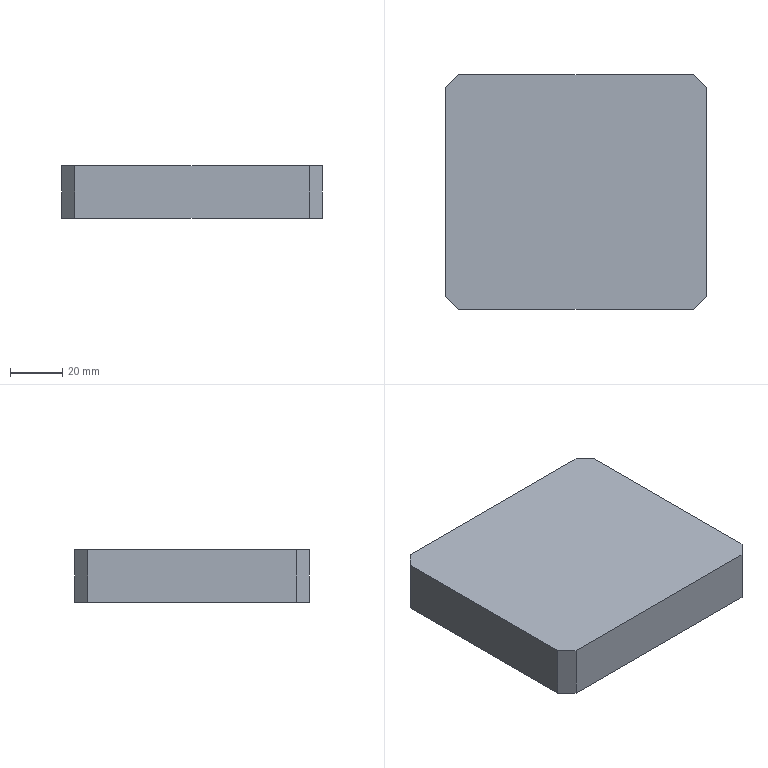Part | SolidWorks | features Chamfer 1, Extrusion 1 | 1 solid | 10 faces | box 100 x 90 x 20 mm | volume 179000 mm3 | plane 10
STEP:
#1=CARTESIAN_POINT('',(-46.616,42.258,0.));
#2=VERTEX_POINT('',#1);
#3=CARTESIAN_POINT('',(-46.616,-37.742,0.));
#4=VERTEX_POINT('',#3);
#5=CARTESIAN_POINT('',(-46.616,47.258,0.));
#6=DIRECTION('',(0.,-1.,0.));
#7=VECTOR('',#6,1000.);
#8=LINE('',#5,#7);
#9=EDGE_CURVE('',#2,#4,#8,.T.);
#10=ORIENTED_EDGE('',*,*,#9,.T.);
#11=CARTESIAN_POINT('',(-46.616,-37.742,20.));
#12=VERTEX_POINT('',#11);
#13=CARTESIAN_POINT('',(-46.616,-37.742,20.));
#14=DIRECTION('',(0.,0.,1.));
#15=VECTOR('',#14,1000.);
#16=LINE('',#13,#15);
#17=EDGE_CURVE('',#4,#12,#16,.T.);
#18=ORIENTED_EDGE('',*,*,#17,.T.);
#19=CARTESIAN_POINT('',(-46.616,42.258,20.));
#20=VERTEX_POINT('',#19);
#21=CARTESIAN_POINT('',(-46.616,47.258,20.));
#22=DIRECTION('',(0.,-1.,0.));
#23=VECTOR('',#22,1000.);
#24=LINE('',#21,#23);
#25=EDGE_CURVE('',#20,#12,#24,.T.);
#26=ORIENTED_EDGE('',*,*,#25,.F.);
#27=CARTESIAN_POINT('',(-46.616,42.258,20.));
#28=DIRECTION('',(0.,0.,-1.));
#29=VECTOR('',#28,1000.);
#30=LINE('',#27,#29);
#31=EDGE_CURVE('',#20,#2,#30,.T.);
#32=ORIENTED_EDGE('',*,*,#31,.T.);
#33=EDGE_LOOP('',(#10,#18,#26,#32));
#34=FACE_OUTER_BOUND('',#33,.T.);
#35=CARTESIAN_POINT('',(-46.616,47.258,20.));
#36=DIRECTION('',(1.,0.,0.));
#37=DIRECTION('',(0.,1.,0.));
#38=AXIS2_PLACEMENT_3D('',#35,#36,#37);
#39=PLANE('',#38);
#40=ADVANCED_FACE('',(#34),#39,.F.);
#41=CARTESIAN_POINT('',(-41.616,-42.742,0.));
#42=VERTEX_POINT('',#41);
#43=CARTESIAN_POINT('',(48.384,-42.742,0.));
#44=VERTEX_POINT('',#43);
#45=CARTESIAN_POINT('',(-46.616,-42.742,0.));
#46=DIRECTION('',(1.,0.,0.));
#47=VECTOR('',#46,1000.);
#48=LINE('',#45,#47);
#49=EDGE_CURVE('',#42,#44,#48,.T.);
#50=ORIENTED_EDGE('',*,*,#49,.T.);
#51=CARTESIAN_POINT('',(48.384,-42.742,20.));
#52=VERTEX_POINT('',#51);
#53=CARTESIAN_POINT('',(48.384,-42.742,20.));
#54=DIRECTION('',(0.,0.,1.));
#55=VECTOR('',#54,1000.);
#56=LINE('',#53,#55);
#57=EDGE_CURVE('',#44,#52,#56,.T.);
#58=ORIENTED_EDGE('',*,*,#57,.T.);
#59=CARTESIAN_POINT('',(-41.616,-42.742,20.));
#60=VERTEX_POINT('',#59);
#61=CARTESIAN_POINT('',(-46.616,-42.742,20.));
#62=DIRECTION('',(1.,0.,0.));
#63=VECTOR('',#62,1000.);
#64=LINE('',#61,#63);
#65=EDGE_CURVE('',#60,#52,#64,.T.);
#66=ORIENTED_EDGE('',*,*,#65,.F.);
#67=CARTESIAN_POINT('',(-41.616,-42.742,20.));
#68=DIRECTION('',(0.,0.,-1.));
#69=VECTOR('',#68,1000.);
#70=LINE('',#67,#69);
#71=EDGE_CURVE('',#60,#42,#70,.T.);
#72=ORIENTED_EDGE('',*,*,#71,.T.);
#73=EDGE_LOOP('',(#50,#58,#66,#72));
#74=FACE_OUTER_BOUND('',#73,.T.);
#75=CARTESIAN_POINT('',(-46.616,-42.742,20.));
#76=DIRECTION('',(0.,1.,0.));
#77=DIRECTION('',(0.,0.,1.));
#78=AXIS2_PLACEMENT_3D('',#75,#76,#77);
#79=PLANE('',#78);
#80=ADVANCED_FACE('',(#74),#79,.F.);
#81=CARTESIAN_POINT('',(53.384,-37.742,20.));
#82=VERTEX_POINT('',#81);
#83=CARTESIAN_POINT('',(53.384,42.258,20.));
#84=VERTEX_POINT('',#83);
#85=CARTESIAN_POINT('',(53.384,47.258,20.));
#86=DIRECTION('',(0.,1.,0.));
#87=VECTOR('',#86,1000.);
#88=LINE('',#85,#87);
#89=EDGE_CURVE('',#82,#84,#88,.T.);
#90=ORIENTED_EDGE('',*,*,#89,.F.);
#91=CARTESIAN_POINT('',(53.384,-37.742,0.));
#92=VERTEX_POINT('',#91);
#93=CARTESIAN_POINT('',(53.384,-37.742,20.));
#94=DIRECTION('',(0.,0.,-1.));
#95=VECTOR('',#94,1000.);
#96=LINE('',#93,#95);
#97=EDGE_CURVE('',#82,#92,#96,.T.);
#98=ORIENTED_EDGE('',*,*,#97,.T.);
#99=CARTESIAN_POINT('',(53.384,42.258,0.));
#100=VERTEX_POINT('',#99);
#101=CARTESIAN_POINT('',(53.384,47.258,0.));
#102=DIRECTION('',(0.,1.,0.));
#103=VECTOR('',#102,1000.);
#104=LINE('',#101,#103);
#105=EDGE_CURVE('',#92,#100,#104,.T.);
#106=ORIENTED_EDGE('',*,*,#105,.T.);
#107=CARTESIAN_POINT('',(53.384,42.258,20.));
#108=DIRECTION('',(0.,0.,1.));
#109=VECTOR('',#108,1000.);
#110=LINE('',#107,#109);
#111=EDGE_CURVE('',#100,#84,#110,.T.);
#112=ORIENTED_EDGE('',*,*,#111,.T.);
#113=EDGE_LOOP('',(#90,#98,#106,#112));
#114=FACE_OUTER_BOUND('',#113,.T.);
#115=CARTESIAN_POINT('',(53.384,47.258,20.));
#116=DIRECTION('',(-1.,0.,0.));
#117=DIRECTION('',(0.,-1.,0.));
#118=AXIS2_PLACEMENT_3D('',#115,#116,#117);
#119=PLANE('',#118);
#120=ADVANCED_FACE('',(#114),#119,.F.);
#121=CARTESIAN_POINT('',(48.384,47.258,0.));
#122=VERTEX_POINT('',#121);
#123=CARTESIAN_POINT('',(-41.616,47.258,0.));
#124=VERTEX_POINT('',#123);
#125=CARTESIAN_POINT('',(-46.616,47.258,0.));
#126=DIRECTION('',(-1.,0.,0.));
#127=VECTOR('',#126,1000.);
#128=LINE('',#125,#127);
#129=EDGE_CURVE('',#122,#124,#128,.T.);
#130=ORIENTED_EDGE('',*,*,#129,.T.);
#131=CARTESIAN_POINT('',(-41.616,47.258,20.));
#132=VERTEX_POINT('',#131);
#133=CARTESIAN_POINT('',(-41.616,47.258,20.));
#134=DIRECTION('',(0.,0.,1.));
#135=VECTOR('',#134,1000.);
#136=LINE('',#133,#135);
#137=EDGE_CURVE('',#124,#132,#136,.T.);
#138=ORIENTED_EDGE('',*,*,#137,.T.);
#139=CARTESIAN_POINT('',(48.384,47.258,20.));
#140=VERTEX_POINT('',#139);
#141=CARTESIAN_POINT('',(-46.616,47.258,20.));
#142=DIRECTION('',(-1.,0.,0.));
#143=VECTOR('',#142,1000.);
#144=LINE('',#141,#143);
#145=EDGE_CURVE('',#140,#132,#144,.T.);
#146=ORIENTED_EDGE('',*,*,#145,.F.);
#147=CARTESIAN_POINT('',(48.384,47.258,20.));
#148=DIRECTION('',(0.,0.,-1.));
#149=VECTOR('',#148,1000.);
#150=LINE('',#147,#149);
#151=EDGE_CURVE('',#140,#122,#150,.T.);
#152=ORIENTED_EDGE('',*,*,#151,.T.);
#153=EDGE_LOOP('',(#130,#138,#146,#152));
#154=FACE_OUTER_BOUND('',#153,.T.);
#155=CARTESIAN_POINT('',(-46.616,47.258,20.));
#156=DIRECTION('',(0.,-1.,0.));
#157=DIRECTION('',(0.,0.,-1.));
#158=AXIS2_PLACEMENT_3D('',#155,#156,#157);
#159=PLANE('',#158);
#160=ADVANCED_FACE('',(#154),#159,.F.);
#161=ORIENTED_EDGE('',*,*,#65,.T.);
#162=CARTESIAN_POINT('',(45.563,-45.563,20.));
#163=DIRECTION('',(0.7071,0.7071,0.));
#164=VECTOR('',#163,1000.);
#165=LINE('',#162,#164);
#166=EDGE_CURVE('',#52,#82,#165,.T.);
#167=ORIENTED_EDGE('',*,*,#166,.T.);
#168=ORIENTED_EDGE('',*,*,#89,.T.);
#169=CARTESIAN_POINT('',(47.821,47.821,20.));
#170=DIRECTION('',(-0.7071,0.7071,0.));
#171=VECTOR('',#170,1000.);
#172=LINE('',#169,#171);
#173=EDGE_CURVE('',#84,#140,#172,.T.);
#174=ORIENTED_EDGE('',*,*,#173,.T.);
#175=ORIENTED_EDGE('',*,*,#145,.T.);
#176=CARTESIAN_POINT('',(-44.437,44.437,20.));
#177=DIRECTION('',(-0.7071,-0.7071,0.));
#178=VECTOR('',#177,1000.);
#179=LINE('',#176,#178);
#180=EDGE_CURVE('',#132,#20,#179,.T.);
#181=ORIENTED_EDGE('',*,*,#180,.T.);
#182=ORIENTED_EDGE('',*,*,#25,.T.);
#183=CARTESIAN_POINT('',(-42.179,-42.179,20.));
#184=DIRECTION('',(0.7071,-0.7071,0.));
#185=VECTOR('',#184,1000.);
#186=LINE('',#183,#185);
#187=EDGE_CURVE('',#12,#60,#186,.T.);
#188=ORIENTED_EDGE('',*,*,#187,.T.);
#189=EDGE_LOOP('',(#161,#167,#168,#174,#175,#181,#182,#188));
#190=FACE_OUTER_BOUND('',#189,.T.);
#191=CARTESIAN_POINT('',(0.,0.,20.));
#192=DIRECTION('',(0.,0.,1.));
#193=DIRECTION('',(1.,0.,0.));
#194=AXIS2_PLACEMENT_3D('',#191,#192,#193);
#195=PLANE('',#194);
#196=ADVANCED_FACE('',(#190),#195,.T.);
#197=ORIENTED_EDGE('',*,*,#105,.F.);
#198=CARTESIAN_POINT('',(53.384,-37.742,0.));
#199=DIRECTION('',(-0.7071,-0.7071,0.));
#200=VECTOR('',#199,1000.);
#201=LINE('',#198,#200);
#202=EDGE_CURVE('',#92,#44,#201,.T.);
#203=ORIENTED_EDGE('',*,*,#202,.T.);
#204=ORIENTED_EDGE('',*,*,#49,.F.);
#205=CARTESIAN_POINT('',(-41.616,-42.742,0.));
#206=DIRECTION('',(-0.7071,0.7071,0.));
#207=VECTOR('',#206,1000.);
#208=LINE('',#205,#207);
#209=EDGE_CURVE('',#42,#4,#208,.T.);
#210=ORIENTED_EDGE('',*,*,#209,.T.);
#211=ORIENTED_EDGE('',*,*,#9,.F.);
#212=CARTESIAN_POINT('',(-46.616,42.258,0.));
#213=DIRECTION('',(0.7071,0.7071,0.));
#214=VECTOR('',#213,1000.);
#215=LINE('',#212,#214);
#216=EDGE_CURVE('',#2,#124,#215,.T.);
#217=ORIENTED_EDGE('',*,*,#216,.T.);
#218=ORIENTED_EDGE('',*,*,#129,.F.);
#219=CARTESIAN_POINT('',(48.384,47.258,0.));
#220=DIRECTION('',(0.7071,-0.7071,0.));
#221=VECTOR('',#220,1000.);
#222=LINE('',#219,#221);
#223=EDGE_CURVE('',#122,#100,#222,.T.);
#224=ORIENTED_EDGE('',*,*,#223,.T.);
#225=EDGE_LOOP('',(#197,#203,#204,#210,#211,#217,#218,#224));
#226=FACE_OUTER_BOUND('',#225,.T.);
#227=CARTESIAN_POINT('',(0.,0.,0.));
#228=DIRECTION('',(0.,0.,1.));
#229=DIRECTION('',(1.,0.,0.));
#230=AXIS2_PLACEMENT_3D('',#227,#228,#229);
#231=PLANE('',#230);
#232=ADVANCED_FACE('',(#226),#231,.F.);
#233=ORIENTED_EDGE('',*,*,#166,.F.);
#234=ORIENTED_EDGE('',*,*,#57,.F.);
#235=ORIENTED_EDGE('',*,*,#202,.F.);
#236=ORIENTED_EDGE('',*,*,#97,.F.);
#237=EDGE_LOOP('',(#233,#234,#235,#236));
#238=FACE_OUTER_BOUND('',#237,.T.);
#239=CARTESIAN_POINT('',(53.384,-37.742,20.));
#240=DIRECTION('',(-0.7071,0.7071,0.));
#241=DIRECTION('',(0.,0.,-1.));
#242=AXIS2_PLACEMENT_3D('',#239,#240,#241);
#243=PLANE('',#242);
#244=ADVANCED_FACE('',(#238),#243,.F.);
#245=ORIENTED_EDGE('',*,*,#187,.F.);
#246=ORIENTED_EDGE('',*,*,#17,.F.);
#247=ORIENTED_EDGE('',*,*,#209,.F.);
#248=ORIENTED_EDGE('',*,*,#71,.F.);
#249=EDGE_LOOP('',(#245,#246,#247,#248));
#250=FACE_OUTER_BOUND('',#249,.T.);
#251=CARTESIAN_POINT('',(-41.616,-42.742,20.));
#252=DIRECTION('',(0.7071,0.7071,0.));
#253=DIRECTION('',(0.,0.,-1.));
#254=AXIS2_PLACEMENT_3D('',#251,#252,#253);
#255=PLANE('',#254);
#256=ADVANCED_FACE('',(#250),#255,.F.);
#257=ORIENTED_EDGE('',*,*,#180,.F.);
#258=ORIENTED_EDGE('',*,*,#137,.F.);
#259=ORIENTED_EDGE('',*,*,#216,.F.);
#260=ORIENTED_EDGE('',*,*,#31,.F.);
#261=EDGE_LOOP('',(#257,#258,#259,#260));
#262=FACE_OUTER_BOUND('',#261,.T.);
#263=CARTESIAN_POINT('',(-46.616,42.258,20.));
#264=DIRECTION('',(0.7071,-0.7071,0.));
#265=DIRECTION('',(0.,0.,-1.));
#266=AXIS2_PLACEMENT_3D('',#263,#264,#265);
#267=PLANE('',#266);
#268=ADVANCED_FACE('',(#262),#267,.F.);
#269=ORIENTED_EDGE('',*,*,#173,.F.);
#270=ORIENTED_EDGE('',*,*,#111,.F.);
#271=ORIENTED_EDGE('',*,*,#223,.F.);
#272=ORIENTED_EDGE('',*,*,#151,.F.);
#273=EDGE_LOOP('',(#269,#270,#271,#272));
#274=FACE_OUTER_BOUND('',#273,.T.);
#275=CARTESIAN_POINT('',(48.384,47.258,20.));
#276=DIRECTION('',(-0.7071,-0.7071,0.));
#277=DIRECTION('',(0.,0.,-1.));
#278=AXIS2_PLACEMENT_3D('',#275,#276,#277);
#279=PLANE('',#278);
#280=ADVANCED_FACE('',(#274),#279,.F.);
#281=CLOSED_SHELL('',(#40,#80,#120,#160,#196,#232,#244,#256,#268,#280));
#282=MANIFOLD_SOLID_BREP('',#281);
#283=CARTESIAN_POINT('',(0.,0.,0.));
#284=DIRECTION('',(0.,0.,1.));
#285=DIRECTION('',(1.,0.,0.));
#286=AXIS2_PLACEMENT_3D('',#283,#284,#285);
#287=(LENGTH_UNIT()NAMED_UNIT(*)SI_UNIT(.MILLI.,.METRE.));
#288=UNCERTAINTY_MEASURE_WITH_UNIT(LENGTH_MEASURE(0.00001),#287,'','');
#289=(NAMED_UNIT(*)PLANE_ANGLE_UNIT()SI_UNIT($,.RADIAN.));
#290=(NAMED_UNIT(*)SI_UNIT($,.STERADIAN.)SOLID_ANGLE_UNIT());
#291=(GEOMETRIC_REPRESENTATION_CONTEXT(3)GLOBAL_UNCERTAINTY_ASSIGNED_CONTEXT((#288))GLOBAL_UNIT_ASSIGNED_CONTEXT((#287,#289,#290))REPRESENTATION_CONTEXT('',''));
#292=ADVANCED_BREP_SHAPE_REPRESENTATION('',(#282,#286),#291);